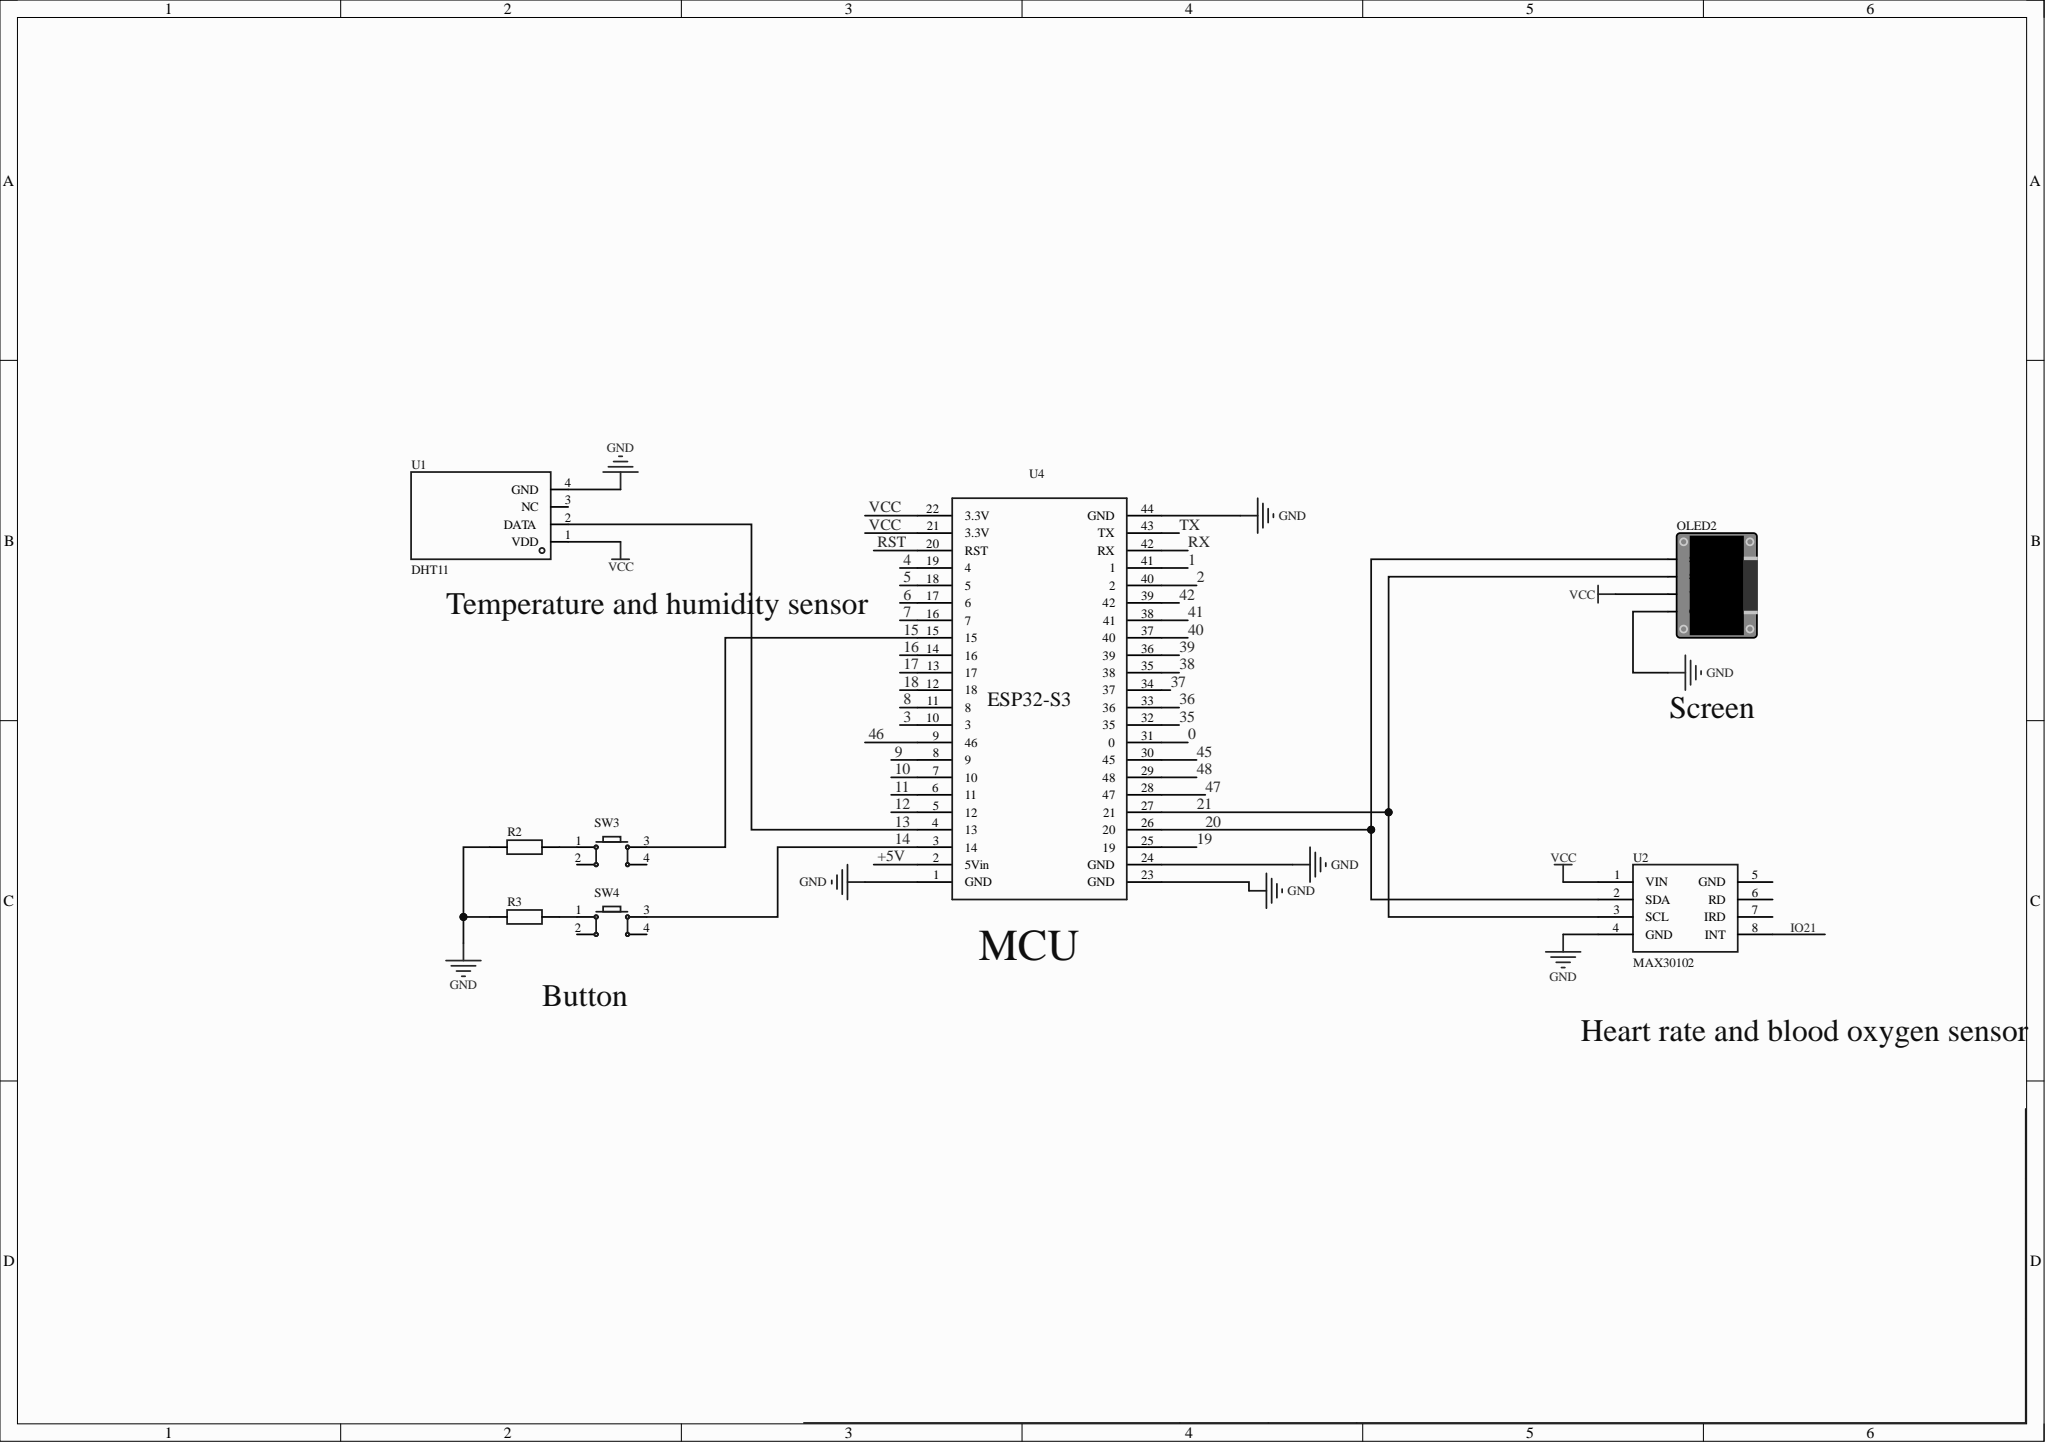Circuit board | Altium Designer | 8 parts | 9 nets
Bill of materials:
Comment,Description,Designator,Footprint,LibRef,Quantity
"","","OLED2","0.96OLED_4P","0.96OLED模块_4P","1"
"10K","","R2, R3","R0603","Res_0603","2"
"","","SW3, SW4","SW-TH_4P-L6.0-W6.0-P4.50-LS6.5","Key_TH_6x6x6","2"
"DHT11","New capacitive digital temperature and humidity sensor; old model discontinued; 16.1x12.6x5.8mm","U1","SENSOR-TH_DHT11","DHT11","1"
"MAX30102","","U2","MAX30102","MAX30102","1"
"NO","","U4","ESP32S3","NO","1"
Netlist (Protel format):
[
OLED2
0.96OLED_4P




]
[
R2
R0603
10K



]
[
R3
R0603
10K



]
[
SW3
SW-TH_4P-L6.0-W6.0-P4.50-LS6.5




]
[
SW4
SW-TH_4P-L6.0-W6.0-P4.50-LS6.5




]
[
U1
SENSOR-TH_DHT11
DHT11



]
[
U2
MAX30102
MAX30102



]
[
U4
ESP32S3
NO



]
(
VCC
OLED2-2
U1-1
U2-1
U4-21
U4-22
)
(
NetR3_2
R3-2
SW4-1
)
(
NetR2_2
R2-2
SW3-1
)
(
GND
OLED2-1
R2-1
R3-1
U1-4
U2-4
U4-1
U4-23
U4-24
U4-44
)
(
21
OLED2-3
U2-3
U4-27
)
(
20
OLED2-4
U2-2
U4-26
)
(
15
SW3-3
U4-15
)
(
14
SW4-3
U4-3
)
(
13
U1-2
U4-4
)